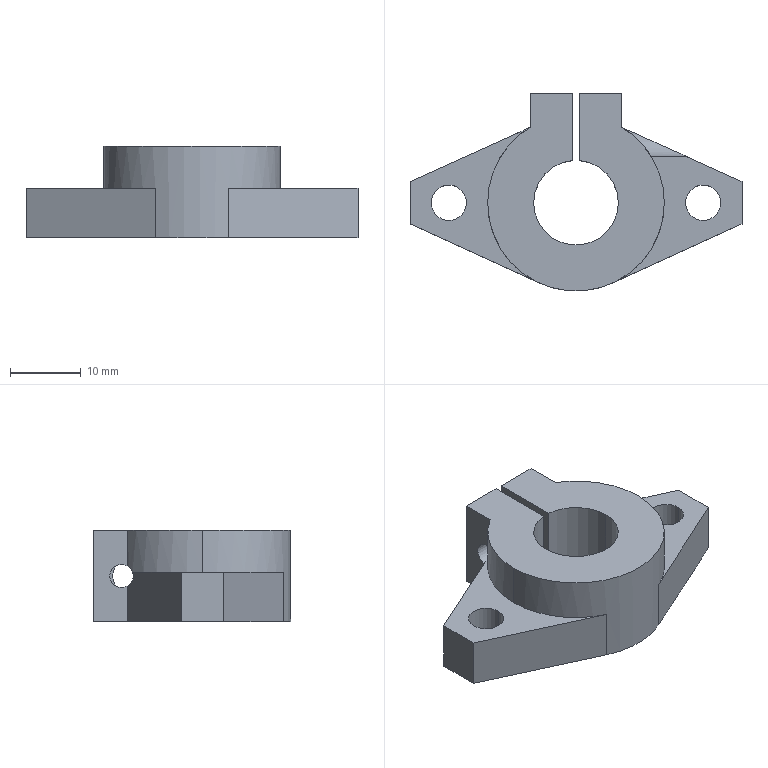Part | SolidWorks | features HoleWzd 2, ICE 2, Extrusion 1 | 1 solid | 33 faces | box 47 x 28 x 13 mm | volume 6727 mm3 | plane 17 | cylinder 16 | commonest cylinder face diameters 5 x4 12 x3 25 x3 3.3 x2 4.5 x2 8 x2
STEP:
#1=CARTESIAN_POINT('',(1.9,10.5,4.));
#2=VERTEX_POINT('',#1);
#3=CARTESIAN_POINT('',(1.9,10.5,-4.));
#4=VERTEX_POINT('',#3);
#5=CARTESIAN_POINT('',(1.9,10.5,0.));
#6=DIRECTION('',(1.,0.,0.));
#7=DIRECTION('',(0.,0.,-1.));
#8=AXIS2_PLACEMENT_3D('',#5,#6,#7);
#9=CIRCLE('',#8,4.);
#10=EDGE_CURVE('',#2,#4,#9,.T.);
#11=ORIENTED_EDGE('',*,*,#10,.F.);
#12=CARTESIAN_POINT('',(6.782,10.5,4.));
#13=VERTEX_POINT('',#12);
#14=CARTESIAN_POINT('',(6.5,10.5,4.));
#15=DIRECTION('',(1.,0.,0.));
#16=VECTOR('',#15,1000.);
#17=LINE('',#14,#16);
#18=EDGE_CURVE('',#2,#13,#17,.T.);
#19=ORIENTED_EDGE('',*,*,#18,.T.);
#20=CARTESIAN_POINT('',(10.658,6.531,0.5));
#21=VERTEX_POINT('',#20);
#22=CARTESIAN_POINT('',(6.782,10.5,4.));
#23=CARTESIAN_POINT('',(7.288,10.174,4.));
#24=CARTESIAN_POINT('',(7.763,9.815,3.961));
#25=CARTESIAN_POINT('',(8.43,9.234,3.8));
#26=CARTESIAN_POINT('',(8.647,9.031,3.727));
#27=CARTESIAN_POINT('',(9.053,8.625,3.54));
#28=CARTESIAN_POINT('',(9.242,8.421,3.426));
#29=CARTESIAN_POINT('',(9.594,8.018,3.146));
#30=CARTESIAN_POINT('',(9.756,7.818,2.979));
#31=CARTESIAN_POINT('',(10.04,7.449,2.601));
#32=CARTESIAN_POINT('',(10.164,7.279,2.388));
#33=CARTESIAN_POINT('',(10.323,7.05,2.028));
#34=CARTESIAN_POINT('',(10.371,6.978,1.902));
#35=CARTESIAN_POINT('',(10.456,6.85,1.642));
#36=CARTESIAN_POINT('',(10.494,6.792,1.508));
#37=CARTESIAN_POINT('',(10.558,6.692,1.233));
#38=CARTESIAN_POINT('',(10.585,6.649,1.091));
#39=CARTESIAN_POINT('',(10.629,6.578,0.7995));
#40=CARTESIAN_POINT('',(10.646,6.55,0.6495));
#41=CARTESIAN_POINT('',(10.658,6.531,0.5));
#42=B_SPLINE_CURVE_WITH_KNOTS('',3,(#22,#23,#24,#25,#26,#27,#28,#29,#30,#31,#32,#33,#34,#35,#36,#37,#38,#39,#40,#41),.UNSPECIFIED.,.F.,.F.,(4,2,2,2,2,2,2,2,2,4),(0.0003296,0.002119,0.003014,0.003908,0.004803,0.005698,0.006145,0.006592,0.00704,0.007487),.UNSPECIFIED.);
#43=EDGE_CURVE('',#13,#21,#42,.T.);
#44=ORIENTED_EDGE('',*,*,#43,.T.);
#45=CARTESIAN_POINT('',(15.68,6.531,0.5));
#46=VERTEX_POINT('',#45);
#47=CARTESIAN_POINT('',(16.5,6.531,0.5));
#48=DIRECTION('',(1.,0.,0.));
#49=VECTOR('',#48,1000.);
#50=LINE('',#47,#49);
#51=EDGE_CURVE('',#21,#46,#50,.T.);
#52=ORIENTED_EDGE('',*,*,#51,.T.);
#53=CARTESIAN_POINT('',(6.892,10.5,-4.));
#54=VERTEX_POINT('',#53);
#55=CARTESIAN_POINT('',(15.68,6.531,0.5));
#56=CARTESIAN_POINT('',(16.395,6.208,-2.063));
#57=CARTESIAN_POINT('',(12.612,7.917,-4.));
#58=CARTESIAN_POINT('',(6.892,10.5,-4.));
#59=(BOUNDED_CURVE()B_SPLINE_CURVE(3,(#55,#56,#57,#58),.UNSPECIFIED.,.F.,.F.)B_SPLINE_CURVE_WITH_KNOTS((4,4),(3.016,4.712),.UNSPECIFIED.)CURVE()GEOMETRIC_REPRESENTATION_ITEM()RATIONAL_B_SPLINE_CURVE((1.,0.7743,0.7743,1.))REPRESENTATION_ITEM(''));
#60=EDGE_CURVE('',#46,#54,#59,.T.);
#61=ORIENTED_EDGE('',*,*,#60,.T.);
#62=CARTESIAN_POINT('',(6.5,10.5,-4.));
#63=DIRECTION('',(1.,0.,0.));
#64=VECTOR('',#63,1000.);
#65=LINE('',#62,#64);
#66=EDGE_CURVE('',#4,#54,#65,.T.);
#67=ORIENTED_EDGE('',*,*,#66,.F.);
#68=EDGE_LOOP('',(#11,#19,#44,#52,#61,#67));
#69=FACE_OUTER_BOUND('',#68,.T.);
#70=CARTESIAN_POINT('',(6.5,10.5,0.));
#71=DIRECTION('',(1.,0.,0.));
#72=DIRECTION('',(0.,0.,-1.));
#73=AXIS2_PLACEMENT_3D('',#70,#71,#72);
#74=CYLINDRICAL_SURFACE('',#73,4.);
#75=ADVANCED_FACE('',(#69),#74,.F.);
#76=CARTESIAN_POINT('',(0.5,10.5,2.25));
#77=VERTEX_POINT('',#76);
#78=CARTESIAN_POINT('',(0.5,10.5,-2.25));
#79=VERTEX_POINT('',#78);
#80=CARTESIAN_POINT('',(0.5,10.5,0.));
#81=DIRECTION('',(1.,0.,0.));
#82=DIRECTION('',(0.,0.,-1.));
#83=AXIS2_PLACEMENT_3D('',#80,#81,#82);
#84=CIRCLE('',#83,2.25);
#85=EDGE_CURVE('',#77,#79,#84,.T.);
#86=ORIENTED_EDGE('',*,*,#85,.F.);
#87=CARTESIAN_POINT('',(1.9,10.5,2.25));
#88=VERTEX_POINT('',#87);
#89=CARTESIAN_POINT('',(6.5,10.5,2.25));
#90=DIRECTION('',(1.,0.,0.));
#91=VECTOR('',#90,1000.);
#92=LINE('',#89,#91);
#93=EDGE_CURVE('',#77,#88,#92,.T.);
#94=ORIENTED_EDGE('',*,*,#93,.T.);
#95=CARTESIAN_POINT('',(1.9,10.5,-2.25));
#96=VERTEX_POINT('',#95);
#97=CARTESIAN_POINT('',(1.9,10.5,0.));
#98=DIRECTION('',(1.,0.,0.));
#99=DIRECTION('',(0.,0.,-1.));
#100=AXIS2_PLACEMENT_3D('',#97,#98,#99);
#101=CIRCLE('',#100,2.25);
#102=EDGE_CURVE('',#88,#96,#101,.T.);
#103=ORIENTED_EDGE('',*,*,#102,.T.);
#104=CARTESIAN_POINT('',(6.5,10.5,-2.25));
#105=DIRECTION('',(1.,0.,0.));
#106=VECTOR('',#105,1000.);
#107=LINE('',#104,#106);
#108=EDGE_CURVE('',#79,#96,#107,.T.);
#109=ORIENTED_EDGE('',*,*,#108,.F.);
#110=EDGE_LOOP('',(#86,#94,#103,#109));
#111=FACE_OUTER_BOUND('',#110,.T.);
#112=CARTESIAN_POINT('',(6.5,10.5,0.));
#113=DIRECTION('',(1.,0.,0.));
#114=DIRECTION('',(0.,0.,-1.));
#115=AXIS2_PLACEMENT_3D('',#112,#113,#114);
#116=CYLINDRICAL_SURFACE('',#115,2.25);
#117=ADVANCED_FACE('',(#111),#116,.F.);
#118=CARTESIAN_POINT('',(-6.5,11.5,1.65));
#119=VERTEX_POINT('',#118);
#120=CARTESIAN_POINT('',(-6.5,10.677,1.43));
#121=VERTEX_POINT('',#120);
#122=CARTESIAN_POINT('',(-6.5,11.5,0.));
#123=DIRECTION('',(1.,0.,0.));
#124=DIRECTION('',(0.,1.,0.));
#125=AXIS2_PLACEMENT_3D('',#122,#123,#124);
#126=CIRCLE('',#125,1.65);
#127=EDGE_CURVE('',#119,#121,#126,.T.);
#128=ORIENTED_EDGE('',*,*,#127,.F.);
#129=CARTESIAN_POINT('',(-0.5,11.5,1.65));
#130=VERTEX_POINT('',#129);
#131=CARTESIAN_POINT('',(-0.5,11.5,1.65));
#132=DIRECTION('',(1.,0.,0.));
#133=VECTOR('',#132,1000.);
#134=LINE('',#131,#133);
#135=EDGE_CURVE('',#119,#130,#134,.T.);
#136=ORIENTED_EDGE('',*,*,#135,.T.);
#137=CARTESIAN_POINT('',(-0.5,11.5,-1.65));
#138=VERTEX_POINT('',#137);
#139=CARTESIAN_POINT('',(-0.5,11.5,0.));
#140=DIRECTION('',(1.,0.,0.));
#141=DIRECTION('',(0.,0.,-1.));
#142=AXIS2_PLACEMENT_3D('',#139,#140,#141);
#143=CIRCLE('',#142,1.65);
#144=EDGE_CURVE('',#130,#138,#143,.T.);
#145=ORIENTED_EDGE('',*,*,#144,.T.);
#146=CARTESIAN_POINT('',(-6.5,11.5,-1.65));
#147=VERTEX_POINT('',#146);
#148=CARTESIAN_POINT('',(-0.5,11.5,-1.65));
#149=DIRECTION('',(1.,0.,0.));
#150=VECTOR('',#149,1000.);
#151=LINE('',#148,#150);
#152=EDGE_CURVE('',#147,#138,#151,.T.);
#153=ORIENTED_EDGE('',*,*,#152,.F.);
#154=CARTESIAN_POINT('',(-6.5,10.677,-1.43));
#155=VERTEX_POINT('',#154);
#156=CARTESIAN_POINT('',(-6.5,11.5,0.));
#157=DIRECTION('',(1.,0.,0.));
#158=DIRECTION('',(0.,1.,0.));
#159=AXIS2_PLACEMENT_3D('',#156,#157,#158);
#160=CIRCLE('',#159,1.65);
#161=EDGE_CURVE('',#155,#147,#160,.T.);
#162=ORIENTED_EDGE('',*,*,#161,.F.);
#163=CARTESIAN_POINT('',(-8.16,9.928,0.5));
#164=VERTEX_POINT('',#163);
#165=CARTESIAN_POINT('',(-6.5,10.677,-1.43));
#166=CARTESIAN_POINT('',(-8.054,9.975,-1.026));
#167=CARTESIAN_POINT('',(-8.703,9.682,-0.2716));
#168=CARTESIAN_POINT('',(-8.16,9.928,0.5));
#169=(BOUNDED_CURVE()B_SPLINE_CURVE(3,(#165,#166,#167,#168),.UNSPECIFIED.,.F.,.F.)B_SPLINE_CURVE_WITH_KNOTS((4,4),(2.093,3.449),.UNSPECIFIED.)CURVE()GEOMETRIC_REPRESENTATION_ITEM()RATIONAL_B_SPLINE_CURVE((1.,0.8524,0.8524,1.))REPRESENTATION_ITEM(''));
#170=EDGE_CURVE('',#155,#164,#169,.T.);
#171=ORIENTED_EDGE('',*,*,#170,.T.);
#172=CARTESIAN_POINT('',(-7.596,9.928,0.5));
#173=VERTEX_POINT('',#172);
#174=CARTESIAN_POINT('',(-0.5,9.928,0.5));
#175=DIRECTION('',(-1.,0.,0.));
#176=VECTOR('',#175,1000.);
#177=LINE('',#174,#176);
#178=EDGE_CURVE('',#173,#164,#177,.T.);
#179=ORIENTED_EDGE('',*,*,#178,.F.);
#180=CARTESIAN_POINT('',(-6.5,10.677,1.43));
#181=CARTESIAN_POINT('',(-6.728,10.538,1.35));
#182=CARTESIAN_POINT('',(-6.941,10.398,1.245));
#183=CARTESIAN_POINT('',(-7.23,10.197,1.018));
#184=CARTESIAN_POINT('',(-7.319,10.134,0.9323));
#185=CARTESIAN_POINT('',(-7.476,10.018,0.7346));
#186=CARTESIAN_POINT('',(-7.544,9.967,0.623));
#187=CARTESIAN_POINT('',(-7.596,9.928,0.5));
#188=B_SPLINE_CURVE_WITH_KNOTS('',3,(#180,#181,#182,#183,#184,#185,#186,#187),.UNSPECIFIED.,.F.,.F.,(4,2,2,4),(0.,0.0008278,0.001242,0.001656),.UNSPECIFIED.);
#189=EDGE_CURVE('',#121,#173,#188,.T.);
#190=ORIENTED_EDGE('',*,*,#189,.F.);
#191=EDGE_LOOP('',(#128,#136,#145,#153,#162,#171,#179,#190));
#192=FACE_OUTER_BOUND('',#191,.T.);
#193=CARTESIAN_POINT('',(-0.5,11.5,0.));
#194=DIRECTION('',(1.,0.,0.));
#195=DIRECTION('',(0.,0.,-1.));
#196=AXIS2_PLACEMENT_3D('',#193,#194,#195);
#197=CYLINDRICAL_SURFACE('',#196,1.65);
#198=ADVANCED_FACE('',(#192),#197,.F.);
#199=CARTESIAN_POINT('',(-15.5,0.,0.5));
#200=VERTEX_POINT('',#199);
#201=CARTESIAN_POINT('',(-20.5,0.,0.5));
#202=VERTEX_POINT('',#201);
#203=CARTESIAN_POINT('',(-18.,0.,0.5));
#204=DIRECTION('',(0.,0.,-1.));
#205=DIRECTION('',(-1.,0.,0.));
#206=AXIS2_PLACEMENT_3D('',#203,#204,#205);
#207=CIRCLE('',#206,2.5);
#208=EDGE_CURVE('',#200,#202,#207,.T.);
#209=ORIENTED_EDGE('',*,*,#208,.F.);
#210=CARTESIAN_POINT('',(-15.5,0.,-6.5));
#211=VERTEX_POINT('',#210);
#212=CARTESIAN_POINT('',(-15.5,0.,0.5));
#213=DIRECTION('',(0.,0.,-1.));
#214=VECTOR('',#213,1000.);
#215=LINE('',#212,#214);
#216=EDGE_CURVE('',#200,#211,#215,.T.);
#217=ORIENTED_EDGE('',*,*,#216,.T.);
#218=CARTESIAN_POINT('',(-20.5,0.,-6.5));
#219=VERTEX_POINT('',#218);
#220=CARTESIAN_POINT('',(-18.,0.,-6.5));
#221=DIRECTION('',(0.,0.,-1.));
#222=DIRECTION('',(-1.,0.,0.));
#223=AXIS2_PLACEMENT_3D('',#220,#221,#222);
#224=CIRCLE('',#223,2.5);
#225=EDGE_CURVE('',#211,#219,#224,.T.);
#226=ORIENTED_EDGE('',*,*,#225,.T.);
#227=CARTESIAN_POINT('',(-20.5,0.,0.5));
#228=DIRECTION('',(0.,0.,-1.));
#229=VECTOR('',#228,1000.);
#230=LINE('',#227,#229);
#231=EDGE_CURVE('',#202,#219,#230,.T.);
#232=ORIENTED_EDGE('',*,*,#231,.F.);
#233=EDGE_LOOP('',(#209,#217,#226,#232));
#234=FACE_OUTER_BOUND('',#233,.T.);
#235=CARTESIAN_POINT('',(-18.,0.,0.5));
#236=DIRECTION('',(0.,0.,-1.));
#237=DIRECTION('',(-1.,0.,0.));
#238=AXIS2_PLACEMENT_3D('',#235,#236,#237);
#239=CYLINDRICAL_SURFACE('',#238,2.5);
#240=ADVANCED_FACE('',(#234),#239,.F.);
#241=CARTESIAN_POINT('',(20.5,0.,0.5));
#242=VERTEX_POINT('',#241);
#243=CARTESIAN_POINT('',(15.5,0.,0.5));
#244=VERTEX_POINT('',#243);
#245=CARTESIAN_POINT('',(18.,0.,0.5));
#246=DIRECTION('',(0.,0.,-1.));
#247=DIRECTION('',(-1.,0.,0.));
#248=AXIS2_PLACEMENT_3D('',#245,#246,#247);
#249=CIRCLE('',#248,2.5);
#250=EDGE_CURVE('',#242,#244,#249,.T.);
#251=ORIENTED_EDGE('',*,*,#250,.F.);
#252=CARTESIAN_POINT('',(20.5,0.,-6.5));
#253=VERTEX_POINT('',#252);
#254=CARTESIAN_POINT('',(20.5,0.,0.5));
#255=DIRECTION('',(0.,0.,-1.));
#256=VECTOR('',#255,1000.);
#257=LINE('',#254,#256);
#258=EDGE_CURVE('',#242,#253,#257,.T.);
#259=ORIENTED_EDGE('',*,*,#258,.T.);
#260=CARTESIAN_POINT('',(15.5,0.,-6.5));
#261=VERTEX_POINT('',#260);
#262=CARTESIAN_POINT('',(18.,0.,-6.5));
#263=DIRECTION('',(0.,0.,-1.));
#264=DIRECTION('',(-1.,0.,0.));
#265=AXIS2_PLACEMENT_3D('',#262,#263,#264);
#266=CIRCLE('',#265,2.5);
#267=EDGE_CURVE('',#253,#261,#266,.T.);
#268=ORIENTED_EDGE('',*,*,#267,.T.);
#269=CARTESIAN_POINT('',(15.5,0.,0.5));
#270=DIRECTION('',(0.,0.,-1.));
#271=VECTOR('',#270,1000.);
#272=LINE('',#269,#271);
#273=EDGE_CURVE('',#244,#261,#272,.T.);
#274=ORIENTED_EDGE('',*,*,#273,.F.);
#275=EDGE_LOOP('',(#251,#259,#268,#274));
#276=FACE_OUTER_BOUND('',#275,.T.);
#277=CARTESIAN_POINT('',(18.,0.,0.5));
#278=DIRECTION('',(0.,0.,-1.));
#279=DIRECTION('',(-1.,0.,0.));
#280=AXIS2_PLACEMENT_3D('',#277,#278,#279);
#281=CYLINDRICAL_SURFACE('',#280,2.5);
#282=ADVANCED_FACE('',(#276),#281,.F.);
#283=CARTESIAN_POINT('',(6.,0.,6.5));
#284=VERTEX_POINT('',#283);
#285=CARTESIAN_POINT('',(-6.,0.,6.5));
#286=VERTEX_POINT('',#285);
#287=CARTESIAN_POINT('',(0.,0.,6.5));
#288=DIRECTION('',(0.,0.,-1.));
#289=DIRECTION('',(1.,0.,0.));
#290=AXIS2_PLACEMENT_3D('',#287,#288,#289);
#291=CIRCLE('',#290,6.);
#292=EDGE_CURVE('',#284,#286,#291,.T.);
#293=ORIENTED_EDGE('',*,*,#292,.F.);
#294=CARTESIAN_POINT('',(6.,0.,-6.5));
#295=VERTEX_POINT('',#294);
#296=CARTESIAN_POINT('',(6.,0.,6.5));
#297=DIRECTION('',(0.,0.,-1.));
#298=VECTOR('',#297,1000.);
#299=LINE('',#296,#298);
#300=EDGE_CURVE('',#284,#295,#299,.T.);
#301=ORIENTED_EDGE('',*,*,#300,.T.);
#302=CARTESIAN_POINT('',(-6.,0.,-6.5));
#303=VERTEX_POINT('',#302);
#304=CARTESIAN_POINT('',(0.,0.,-6.5));
#305=DIRECTION('',(0.,0.,-1.));
#306=DIRECTION('',(1.,0.,0.));
#307=AXIS2_PLACEMENT_3D('',#304,#305,#306);
#308=CIRCLE('',#307,6.);
#309=EDGE_CURVE('',#295,#303,#308,.T.);
#310=ORIENTED_EDGE('',*,*,#309,.T.);
#311=CARTESIAN_POINT('',(-6.,0.,6.5));
#312=DIRECTION('',(0.,0.,-1.));
#313=VECTOR('',#312,1000.);
#314=LINE('',#311,#313);
#315=EDGE_CURVE('',#286,#303,#314,.T.);
#316=ORIENTED_EDGE('',*,*,#315,.F.);
#317=EDGE_LOOP('',(#293,#301,#310,#316));
#318=FACE_OUTER_BOUND('',#317,.T.);
#319=CARTESIAN_POINT('',(0.,0.,6.5));
#320=DIRECTION('',(0.,0.,-1.));
#321=DIRECTION('',(-1.,0.,0.));
#322=AXIS2_PLACEMENT_3D('',#319,#320,#321);
#323=CYLINDRICAL_SURFACE('',#322,6.);
#324=ADVANCED_FACE('',(#318),#323,.F.);
#325=CARTESIAN_POINT('',(-0.5,5.979,6.5));
#326=VERTEX_POINT('',#325);
#327=CARTESIAN_POINT('',(0.,0.,6.5));
#328=DIRECTION('',(0.,0.,-1.));
#329=DIRECTION('',(1.,0.,0.));
#330=AXIS2_PLACEMENT_3D('',#327,#328,#329);
#331=CIRCLE('',#330,6.);
#332=EDGE_CURVE('',#286,#326,#331,.T.);
#333=ORIENTED_EDGE('',*,*,#332,.F.);
#334=ORIENTED_EDGE('',*,*,#315,.T.);
#335=CARTESIAN_POINT('',(-0.5,5.979,-6.5));
#336=VERTEX_POINT('',#335);
#337=CARTESIAN_POINT('',(0.,0.,-6.5));
#338=DIRECTION('',(0.,0.,-1.));
#339=DIRECTION('',(1.,0.,0.));
#340=AXIS2_PLACEMENT_3D('',#337,#338,#339);
#341=CIRCLE('',#340,6.);
#342=EDGE_CURVE('',#303,#336,#341,.T.);
#343=ORIENTED_EDGE('',*,*,#342,.T.);
#344=CARTESIAN_POINT('',(-0.5,5.979,6.5));
#345=DIRECTION('',(0.,0.,-1.));
#346=VECTOR('',#345,1000.);
#347=LINE('',#344,#346);
#348=EDGE_CURVE('',#326,#336,#347,.T.);
#349=ORIENTED_EDGE('',*,*,#348,.F.);
#350=EDGE_LOOP('',(#333,#334,#343,#349));
#351=FACE_OUTER_BOUND('',#350,.T.);
#352=CARTESIAN_POINT('',(0.,0.,6.5));
#353=DIRECTION('',(0.,0.,-1.));
#354=DIRECTION('',(-1.,0.,0.));
#355=AXIS2_PLACEMENT_3D('',#352,#353,#354);
#356=CYLINDRICAL_SURFACE('',#355,6.);
#357=ADVANCED_FACE('',(#351),#356,.F.);
#358=CARTESIAN_POINT('',(12.5,0.,6.5));
#359=VERTEX_POINT('',#358);
#360=CARTESIAN_POINT('',(6.5,10.677,6.5));
#361=VERTEX_POINT('',#360);
#362=CARTESIAN_POINT('',(0.,0.,6.5));
#363=DIRECTION('',(0.,0.,1.));
#364=DIRECTION('',(1.,0.,0.));
#365=AXIS2_PLACEMENT_3D('',#362,#363,#364);
#366=CIRCLE('',#365,12.5);
#367=EDGE_CURVE('',#359,#361,#366,.T.);
#368=ORIENTED_EDGE('',*,*,#367,.F.);
#369=CARTESIAN_POINT('',(12.5,0.,0.5));
#370=VERTEX_POINT('',#369);
#371=CARTESIAN_POINT('',(12.5,0.,6.5));
#372=DIRECTION('',(0.,0.,-1.));
#373=VECTOR('',#372,1000.);
#374=LINE('',#371,#373);
#375=EDGE_CURVE('',#359,#370,#374,.T.);
#376=ORIENTED_EDGE('',*,*,#375,.T.);
#377=CARTESIAN_POINT('',(0.,0.,0.5));
#378=DIRECTION('',(0.,0.,-1.));
#379=DIRECTION('',(-1.,0.,0.));
#380=AXIS2_PLACEMENT_3D('',#377,#378,#379);
#381=CIRCLE('',#380,12.5);
#382=EDGE_CURVE('',#21,#370,#381,.T.);
#383=ORIENTED_EDGE('',*,*,#382,.F.);
#384=ORIENTED_EDGE('',*,*,#43,.F.);
#385=CARTESIAN_POINT('',(6.5,10.677,3.996));
#386=VERTEX_POINT('',#385);
#387=CARTESIAN_POINT('',(6.5,10.677,3.996));
#388=CARTESIAN_POINT('',(6.595,10.619,3.999));
#389=CARTESIAN_POINT('',(6.689,10.56,4.));
#390=CARTESIAN_POINT('',(6.782,10.5,4.));
#391=B_SPLINE_CURVE_WITH_KNOTS('',3,(#387,#388,#389,#390),.UNSPECIFIED.,.F.,.F.,(4,4),(0.,0.0003296),.UNSPECIFIED.);
#392=EDGE_CURVE('',#386,#13,#391,.T.);
#393=ORIENTED_EDGE('',*,*,#392,.F.);
#394=CARTESIAN_POINT('',(6.5,10.677,6.5));
#395=DIRECTION('',(0.,0.,-1.));
#396=VECTOR('',#395,1000.);
#397=LINE('',#394,#396);
#398=EDGE_CURVE('',#361,#386,#397,.T.);
#399=ORIENTED_EDGE('',*,*,#398,.F.);
#400=EDGE_LOOP('',(#368,#376,#383,#384,#393,#399));
#401=FACE_OUTER_BOUND('',#400,.T.);
#402=CARTESIAN_POINT('',(0.,0.,6.5));
#403=DIRECTION('',(0.,0.,-1.));
#404=DIRECTION('',(-1.,0.,0.));
#405=AXIS2_PLACEMENT_3D('',#402,#403,#404);
#406=CYLINDRICAL_SURFACE('',#405,12.5);
#407=ADVANCED_FACE('',(#401),#406,.T.);
#408=ORIENTED_EDGE('',*,*,#375,.F.);
#409=CARTESIAN_POINT('',(-12.5,0.,6.5));
#410=VERTEX_POINT('',#409);
#411=CARTESIAN_POINT('',(0.,0.,6.5));
#412=DIRECTION('',(0.,0.,1.));
#413=DIRECTION('',(1.,0.,0.));
#414=AXIS2_PLACEMENT_3D('',#411,#412,#413);
#415=CIRCLE('',#414,12.5);
#416=EDGE_CURVE('',#410,#359,#415,.T.);
#417=ORIENTED_EDGE('',*,*,#416,.F.);
#418=CARTESIAN_POINT('',(-12.5,0.,0.5));
#419=VERTEX_POINT('',#418);
#420=CARTESIAN_POINT('',(-12.5,0.,6.5));
#421=DIRECTION('',(0.,0.,-1.));
#422=VECTOR('',#421,1000.);
#423=LINE('',#420,#422);
#424=EDGE_CURVE('',#410,#419,#423,.T.);
#425=ORIENTED_EDGE('',*,*,#424,.T.);
#426=CARTESIAN_POINT('',(-5.198,-11.368,0.5));
#427=VERTEX_POINT('',#426);
#428=CARTESIAN_POINT('',(0.,0.,0.5));
#429=DIRECTION('',(0.,0.,-1.));
#430=DIRECTION('',(-1.,0.,0.));
#431=AXIS2_PLACEMENT_3D('',#428,#429,#430);
#432=CIRCLE('',#431,12.5);
#433=EDGE_CURVE('',#427,#419,#432,.T.);
#434=ORIENTED_EDGE('',*,*,#433,.F.);
#435=CARTESIAN_POINT('',(-5.198,-11.368,-6.5));
#436=VERTEX_POINT('',#435);
#437=CARTESIAN_POINT('',(-5.198,-11.368,0.5));
#438=DIRECTION('',(0.,0.,-1.));
#439=VECTOR('',#438,1000.);
#440=LINE('',#437,#439);
#441=EDGE_CURVE('',#427,#436,#440,.T.);
#442=ORIENTED_EDGE('',*,*,#441,.T.);
#443=CARTESIAN_POINT('',(5.198,-11.368,-6.5));
#444=VERTEX_POINT('',#443);
#445=CARTESIAN_POINT('',(0.,0.,-6.5));
#446=DIRECTION('',(0.,0.,1.));
#447=DIRECTION('',(1.,0.,0.));
#448=AXIS2_PLACEMENT_3D('',#445,#446,#447);
#449=CIRCLE('',#448,12.5);
#450=EDGE_CURVE('',#436,#444,#449,.T.);
#451=ORIENTED_EDGE('',*,*,#450,.T.);
#452=CARTESIAN_POINT('',(5.198,-11.368,0.5));
#453=VERTEX_POINT('',#452);
#454=CARTESIAN_POINT('',(5.198,-11.368,0.5));
#455=DIRECTION('',(0.,0.,-1.));
#456=VECTOR('',#455,1000.);
#457=LINE('',#454,#456);
#458=EDGE_CURVE('',#453,#444,#457,.T.);
#459=ORIENTED_EDGE('',*,*,#458,.F.);
#460=CARTESIAN_POINT('',(0.,0.,0.5));
#461=DIRECTION('',(0.,0.,-1.));
#462=DIRECTION('',(-1.,0.,0.));
#463=AXIS2_PLACEMENT_3D('',#460,#461,#462);
#464=CIRCLE('',#463,12.5);
#465=EDGE_CURVE('',#370,#453,#464,.T.);
#466=ORIENTED_EDGE('',*,*,#465,.F.);
#467=EDGE_LOOP('',(#408,#417,#425,#434,#442,#451,#459,#466));
#468=FACE_OUTER_BOUND('',#467,.T.);
#469=CARTESIAN_POINT('',(0.,0.,6.5));
#470=DIRECTION('',(0.,0.,-1.));
#471=DIRECTION('',(-1.,0.,0.));
#472=AXIS2_PLACEMENT_3D('',#469,#470,#471);
#473=CYLINDRICAL_SURFACE('',#472,12.5);
#474=ADVANCED_FACE('',(#468),#473,.T.);
#475=ORIENTED_EDGE('',*,*,#424,.F.);
#476=CARTESIAN_POINT('',(-6.5,10.677,6.5));
#477=VERTEX_POINT('',#476);
#478=CARTESIAN_POINT('',(0.,0.,6.5));
#479=DIRECTION('',(0.,0.,1.));
#480=DIRECTION('',(1.,0.,0.));
#481=AXIS2_PLACEMENT_3D('',#478,#479,#480);
#482=CIRCLE('',#481,12.5);
#483=EDGE_CURVE('',#477,#410,#482,.T.);
#484=ORIENTED_EDGE('',*,*,#483,.F.);
#485=CARTESIAN_POINT('',(-6.5,10.677,6.5));
#486=DIRECTION('',(0.,0.,-1.));
#487=VECTOR('',#486,1000.);
#488=LINE('',#485,#487);
#489=EDGE_CURVE('',#477,#121,#488,.T.);
#490=ORIENTED_EDGE('',*,*,#489,.T.);
#491=ORIENTED_EDGE('',*,*,#189,.T.);
#492=CARTESIAN_POINT('',(0.,0.,0.5));
#493=DIRECTION('',(0.,0.,-1.));
#494=DIRECTION('',(-1.,0.,0.));
#495=AXIS2_PLACEMENT_3D('',#492,#493,#494);
#496=CIRCLE('',#495,12.5);
#497=EDGE_CURVE('',#419,#173,#496,.T.);
#498=ORIENTED_EDGE('',*,*,#497,.F.);
#499=EDGE_LOOP('',(#475,#484,#490,#491,#498));
#500=FACE_OUTER_BOUND('',#499,.T.);
#501=CARTESIAN_POINT('',(0.,0.,6.5));
#502=DIRECTION('',(0.,0.,-1.));
#503=DIRECTION('',(-1.,0.,0.));
#504=AXIS2_PLACEMENT_3D('',#501,#502,#503);
#505=CYLINDRICAL_SURFACE('',#504,12.5);
#506=ADVANCED_FACE('',(#500),#505,.T.);
#507=ORIENTED_EDGE('',*,*,#60,.F.);
#508=CARTESIAN_POINT('',(23.5,3.,0.5));
#509=VERTEX_POINT('',#508);
#510=CARTESIAN_POINT('',(5.106,11.307,0.5));
#511=DIRECTION('',(-0.9114,0.4116,0.));
#512=VECTOR('',#511,1000.);
#513=LINE('',#510,#512);
#514=EDGE_CURVE('',#509,#46,#513,.T.);
#515=ORIENTED_EDGE('',*,*,#514,.F.);
#516=CARTESIAN_POINT('',(23.5,3.,-6.5));
#517=VERTEX_POINT('',#516);
#518=CARTESIAN_POINT('',(23.5,3.,0.5));
#519=DIRECTION('',(0.,0.,-1.));
#520=VECTOR('',#519,1000.);
#521=LINE('',#518,#520);
#522=EDGE_CURVE('',#509,#517,#521,.T.);
#523=ORIENTED_EDGE('',*,*,#522,.T.);
#524=CARTESIAN_POINT('',(6.5,10.677,-6.5));
#525=VERTEX_POINT('',#524);
#526=CARTESIAN_POINT('',(5.106,11.307,-6.5));
#527=DIRECTION('',(-0.9114,0.4116,0.));
#528=VECTOR('',#527,1000.);
#529=LINE('',#526,#528);
#530=EDGE_CURVE('',#517,#525,#529,.T.);
#531=ORIENTED_EDGE('',*,*,#530,.T.);
#532=CARTESIAN_POINT('',(6.5,10.677,-3.996));
#533=VERTEX_POINT('',#532);
#534=CARTESIAN_POINT('',(6.5,10.677,0.5));
#535=DIRECTION('',(0.,0.,-1.));
#536=VECTOR('',#535,1000.);
#537=LINE('',#534,#536);
#538=EDGE_CURVE('',#533,#525,#537,.T.);
#539=ORIENTED_EDGE('',*,*,#538,.F.);
#540=CARTESIAN_POINT('',(6.892,10.5,-4.));
#541=CARTESIAN_POINT('',(6.761,10.559,-4.));
#542=CARTESIAN_POINT('',(6.631,10.618,-3.999));
#543=CARTESIAN_POINT('',(6.5,10.677,-3.996));
#544=(BOUNDED_CURVE()B_SPLINE_CURVE(3,(#540,#541,#542,#543),.UNSPECIFIED.,.F.,.F.)B_SPLINE_CURVE_WITH_KNOTS((4,4),(4.712,4.757),.UNSPECIFIED.)CURVE()GEOMETRIC_REPRESENTATION_ITEM()RATIONAL_B_SPLINE_CURVE((1.,0.9998,0.9998,1.))REPRESENTATION_ITEM(''));
#545=EDGE_CURVE('',#54,#533,#544,.T.);
#546=ORIENTED_EDGE('',*,*,#545,.F.);
#547=EDGE_LOOP('',(#507,#515,#523,#531,#539,#546));
#548=FACE_OUTER_BOUND('',#547,.T.);
#549=CARTESIAN_POINT('',(5.106,11.307,0.5));
#550=DIRECTION('',(-0.4116,-0.9114,0.));
#551=DIRECTION('',(0.9114,-0.4116,0.));
#552=AXIS2_PLACEMENT_3D('',#549,#550,#551);
#553=PLANE('',#552);
#554=ADVANCED_FACE('',(#548),#553,.F.);
#555=CARTESIAN_POINT('',(18.,0.,0.5));
#556=DIRECTION('',(0.,0.,-1.));
#557=DIRECTION('',(-1.,0.,0.));
#558=AXIS2_PLACEMENT_3D('',#555,#556,#557);
#559=CIRCLE('',#558,2.5);
#560=EDGE_CURVE('',#244,#242,#559,.T.);
#561=ORIENTED_EDGE('',*,*,#560,.T.);
#562=ORIENTED_EDGE('',*,*,#250,.T.);
#563=EDGE_LOOP('',(#561,#562));
#564=FACE_BOUND('',#563,.T.);
#565=ORIENTED_EDGE('',*,*,#51,.F.);
#566=ORIENTED_EDGE('',*,*,#382,.T.);
#567=ORIENTED_EDGE('',*,*,#465,.T.);
#568=CARTESIAN_POINT('',(23.5,-3.,0.5));
#569=VERTEX_POINT('',#568);
#570=CARTESIAN_POINT('',(5.198,-11.368,0.5));
#571=DIRECTION('',(0.9094,0.4158,0.));
#572=VECTOR('',#571,1000.);
#573=LINE('',#570,#572);
#574=EDGE_CURVE('',#453,#569,#573,.T.);
#575=ORIENTED_EDGE('',*,*,#574,.T.);
#576=CARTESIAN_POINT('',(23.5,0.,0.5));
#577=DIRECTION('',(0.,1.,0.));
#578=VECTOR('',#577,1000.);
#579=LINE('',#576,#578);
#580=EDGE_CURVE('',#569,#509,#579,.T.);
#581=ORIENTED_EDGE('',*,*,#580,.T.);
#582=ORIENTED_EDGE('',*,*,#514,.T.);
#583=EDGE_LOOP('',(#565,#566,#567,#575,#581,#582));
#584=FACE_OUTER_BOUND('',#583,.T.);
#585=CARTESIAN_POINT('',(0.,0.,0.5));
#586=DIRECTION('',(0.,0.,-1.));
#587=DIRECTION('',(-1.,0.,0.));
#588=AXIS2_PLACEMENT_3D('',#585,#586,#587);
#589=PLANE('',#588);
#590=ADVANCED_FACE('',(#564,#584),#589,.F.);
#591=ORIENTED_EDGE('',*,*,#300,.F.);
#592=CARTESIAN_POINT('',(0.5,5.979,6.5));
#593=VERTEX_POINT('',#592);
#594=CARTESIAN_POINT('',(0.,0.,6.5));
#595=DIRECTION('',(0.,0.,-1.));
#596=DIRECTION('',(1.,0.,0.));
#597=AXIS2_PLACEMENT_3D('',#594,#595,#596);
#598=CIRCLE('',#597,6.);
#599=EDGE_CURVE('',#593,#284,#598,.T.);
#600=ORIENTED_EDGE('',*,*,#599,.F.);
#601=CARTESIAN_POINT('',(0.5,5.979,-6.5));
#602=VERTEX_POINT('',#601);
#603=CARTESIAN_POINT('',(0.5,5.979,6.5));
#604=DIRECTION('',(0.,0.,-1.));
#605=VECTOR('',#604,1000.);
#606=LINE('',#603,#605);
#607=EDGE_CURVE('',#593,#602,#606,.T.);
#608=ORIENTED_EDGE('',*,*,#607,.T.);
#609=CARTESIAN_POINT('',(0.,0.,-6.5));
#610=DIRECTION('',(0.,0.,-1.));
#611=DIRECTION('',(1.,0.,0.));
#612=AXIS2_PLACEMENT_3D('',#609,#610,#611);
#613=CIRCLE('',#612,6.);
#614=EDGE_CURVE('',#602,#295,#613,.T.);
#615=ORIENTED_EDGE('',*,*,#614,.T.);
#616=EDGE_LOOP('',(#591,#600,#608,#615));
#617=FACE_OUTER_BOUND('',#616,.T.);
#618=CARTESIAN_POINT('',(0.,0.,6.5));
#619=DIRECTION('',(0.,0.,-1.));
#620=DIRECTION('',(-1.,0.,0.));
#621=AXIS2_PLACEMENT_3D('',#618,#619,#620);
#622=CYLINDRICAL_SURFACE('',#621,6.);
#623=ADVANCED_FACE('',(#617),#622,.F.);
#624=CARTESIAN_POINT('',(-0.5,11.5,0.));
#625=DIRECTION('',(1.,0.,0.));
#626=DIRECTION('',(0.,0.,-1.));
#627=AXIS2_PLACEMENT_3D('',#624,#625,#626);
#628=CIRCLE('',#627,1.65);
#629=EDGE_CURVE('',#138,#130,#628,.T.);
#630=ORIENTED_EDGE('',*,*,#629,.F.);
#631=ORIENTED_EDGE('',*,*,#144,.F.);
#632=EDGE_LOOP('',(#630,#631));
#633=FACE_BOUND('',#632,.T.);
#634=CARTESIAN_POINT('',(-0.5,15.5,-6.5));
#635=VERTEX_POINT('',#634);
#636=CARTESIAN_POINT('',(-0.5,5.979,-6.5));
#637=DIRECTION('',(0.,1.,0.));
#638=VECTOR('',#637,1000.);
#639=LINE('',#636,#638);
#640=EDGE_CURVE('',#336,#635,#639,.T.);
#641=ORIENTED_EDGE('',*,*,#640,.T.);
#642=CARTESIAN_POINT('',(-0.5,15.5,6.5));
#643=VERTEX_POINT('',#642);
#644=CARTESIAN_POINT('',(-0.5,15.5,6.5));
#645=DIRECTION('',(0.,0.,-1.));
#646=VECTOR('',#645,1000.);
#647=LINE('',#644,#646);
#648=EDGE_CURVE('',#643,#635,#647,.T.);
#649=ORIENTED_EDGE('',*,*,#648,.F.);
#650=CARTESIAN_POINT('',(-0.5,5.979,6.5));
#651=DIRECTION('',(0.,1.,0.));
#652=VECTOR('',#651,1000.);
#653=LINE('',#650,#652);
#654=EDGE_CURVE('',#326,#643,#653,.T.);
#655=ORIENTED_EDGE('',*,*,#654,.F.);
#656=ORIENTED_EDGE('',*,*,#348,.T.);
#657=EDGE_LOOP('',(#641,#649,#655,#656));
#658=FACE_OUTER_BOUND('',#657,.T.);
#659=CARTESIAN_POINT('',(-0.5,5.979,6.5));
#660=DIRECTION('',(-1.,0.,0.));
#661=DIRECTION('',(0.,-1.,0.));
#662=AXIS2_PLACEMENT_3D('',#659,#660,#661);
#663=PLANE('',#662);
#664=ADVANCED_FACE('',(#633,#658),#663,.F.);
#665=CARTESIAN_POINT('',(-6.5,15.5,-6.5));
#666=VERTEX_POINT('',#665);
#667=CARTESIAN_POINT('',(-6.5,15.5,-6.5));
#668=DIRECTION('',(-1.,0.,0.));
#669=VECTOR('',#668,1000.);
#670=LINE('',#667,#669);
#671=EDGE_CURVE('',#635,#666,#670,.T.);
#672=ORIENTED_EDGE('',*,*,#671,.T.);
#673=CARTESIAN_POINT('',(-6.5,15.5,6.5));
#674=VERTEX_POINT('',#673);
#675=CARTESIAN_POINT('',(-6.5,15.5,6.5));
#676=DIRECTION('',(0.,0.,-1.));
#677=VECTOR('',#676,1000.);
#678=LINE('',#675,#677);
#679=EDGE_CURVE('',#674,#666,#678,.T.);
#680=ORIENTED_EDGE('',*,*,#679,.F.);
#681=CARTESIAN_POINT('',(-6.5,15.5,6.5));
#682=DIRECTION('',(-1.,0.,0.));
#683=VECTOR('',#682,1000.);
#684=LINE('',#681,#683);
#685=EDGE_CURVE('',#643,#674,#684,.T.);
#686=ORIENTED_EDGE('',*,*,#685,.F.);
#687=ORIENTED_EDGE('',*,*,#648,.T.);
#688=EDGE_LOOP('',(#672,#680,#686,#687));
#689=FACE_OUTER_BOUND('',#688,.T.);
#690=CARTESIAN_POINT('',(-6.5,15.5,6.5));
#691=DIRECTION('',(0.,-1.,0.));
#692=DIRECTION('',(0.,0.,-1.));
#693=AXIS2_PLACEMENT_3D('',#690,#691,#692);
#694=PLANE('',#693);
#695=ADVANCED_FACE('',(#689),#694,.F.);
#696=CARTESIAN_POINT('',(-6.5,10.677,-6.5));
#697=VERTEX_POINT('',#696);
#698=CARTESIAN_POINT('',(-6.5,10.677,0.5));
#699=DIRECTION('',(0.,0.,-1.));
#700=VECTOR('',#699,1000.);
#701=LINE('',#698,#700);
#702=EDGE_CURVE('',#155,#697,#701,.T.);
#703=ORIENTED_EDGE('',*,*,#702,.F.);
#704=ORIENTED_EDGE('',*,*,#161,.T.);
#705=CARTESIAN_POINT('',(-6.5,11.5,0.));
#706=DIRECTION('',(1.,0.,0.));
#707=DIRECTION('',(0.,1.,0.));
#708=AXIS2_PLACEMENT_3D('',#705,#706,#707);
#709=CIRCLE('',#708,1.65);
#710=EDGE_CURVE('',#147,#119,#709,.T.);
#711=ORIENTED_EDGE('',*,*,#710,.T.);
#712=ORIENTED_EDGE('',*,*,#127,.T.);
#713=ORIENTED_EDGE('',*,*,#489,.F.);
#714=CARTESIAN_POINT('',(-6.5,15.5,6.5));
#715=DIRECTION('',(0.,-1.,0.));
#716=VECTOR('',#715,1000.);
#717=LINE('',#714,#716);
#718=EDGE_CURVE('',#674,#477,#717,.T.);
#719=ORIENTED_EDGE('',*,*,#718,.F.);
#720=ORIENTED_EDGE('',*,*,#679,.T.);
#721=CARTESIAN_POINT('',(-6.5,15.5,-6.5));
#722=DIRECTION('',(0.,-1.,0.));
#723=VECTOR('',#722,1000.);
#724=LINE('',#721,#723);
#725=EDGE_CURVE('',#666,#697,#724,.T.);
#726=ORIENTED_EDGE('',*,*,#725,.T.);
#727=EDGE_LOOP('',(#703,#704,#711,#712,#713,#719,#720,#726));
#728=FACE_OUTER_BOUND('',#727,.T.);
#729=CARTESIAN_POINT('',(-6.5,15.5,6.5));
#730=DIRECTION('',(1.,0.,0.));
#731=DIRECTION('',(0.,1.,0.));
#732=AXIS2_PLACEMENT_3D('',#729,#730,#731);
#733=PLANE('',#732);
#734=ADVANCED_FACE('',(#728),#733,.F.);
#735=ORIENTED_EDGE('',*,*,#398,.T.);
#736=CARTESIAN_POINT('',(6.5,10.5,0.));
#737=DIRECTION('',(1.,0.,0.));
#738=DIRECTION('',(0.,0.,-1.));
#739=AXIS2_PLACEMENT_3D('',#736,#737,#738);
#740=CIRCLE('',#739,4.);
#741=EDGE_CURVE('',#533,#386,#740,.T.);
#742=ORIENTED_EDGE('',*,*,#741,.F.);
#743=ORIENTED_EDGE('',*,*,#538,.T.);
#744=CARTESIAN_POINT('',(6.5,15.5,-6.5));
#745=VERTEX_POINT('',#744);
#746=CARTESIAN_POINT('',(6.5,15.5,-6.5));
#747=DIRECTION('',(0.,1.,0.));
#748=VECTOR('',#747,1000.);
#749=LINE('',#746,#748);
#750=EDGE_CURVE('',#525,#745,#749,.T.);
#751=ORIENTED_EDGE('',*,*,#750,.T.);
#752=CARTESIAN_POINT('',(6.5,15.5,6.5));
#753=VERTEX_POINT('',#752);
#754=CARTESIAN_POINT('',(6.5,15.5,6.5));
#755=DIRECTION('',(0.,0.,-1.));
#756=VECTOR('',#755,1000.);
#757=LINE('',#754,#756);
#758=EDGE_CURVE('',#753,#745,#757,.T.);
#759=ORIENTED_EDGE('',*,*,#758,.F.);
#760=CARTESIAN_POINT('',(6.5,15.5,6.5));
#761=DIRECTION('',(0.,1.,0.));
#762=VECTOR('',#761,1000.);
#763=LINE('',#760,#762);
#764=EDGE_CURVE('',#361,#753,#763,.T.);
#765=ORIENTED_EDGE('',*,*,#764,.F.);
#766=EDGE_LOOP('',(#735,#742,#743,#751,#759,#765));
#767=FACE_OUTER_BOUND('',#766,.T.);
#768=CARTESIAN_POINT('',(6.5,15.5,6.5));
#769=DIRECTION('',(-1.,0.,0.));
#770=DIRECTION('',(0.,0.,1.));
#771=AXIS2_PLACEMENT_3D('',#768,#769,#770);
#772=PLANE('',#771);
#773=ADVANCED_FACE('',(#767),#772,.F.);
#774=CARTESIAN_POINT('',(0.5,15.5,-6.5));
#775=VERTEX_POINT('',#774);
#776=CARTESIAN_POINT('',(0.5,15.5,-6.5));
#777=DIRECTION('',(-1.,0.,0.));
#778=VECTOR('',#777,1000.);
#779=LINE('',#776,#778);
#780=EDGE_CURVE('',#745,#775,#779,.T.);
#781=ORIENTED_EDGE('',*,*,#780,.T.);
#782=CARTESIAN_POINT('',(0.5,15.5,6.5));
#783=VERTEX_POINT('',#782);
#784=CARTESIAN_POINT('',(0.5,15.5,6.5));
#785=DIRECTION('',(0.,0.,-1.));
#786=VECTOR('',#785,1000.);
#787=LINE('',#784,#786);
#788=EDGE_CURVE('',#783,#775,#787,.T.);
#789=ORIENTED_EDGE('',*,*,#788,.F.);
#790=CARTESIAN_POINT('',(0.5,15.5,6.5));
#791=DIRECTION('',(-1.,0.,0.));
#792=VECTOR('',#791,1000.);
#793=LINE('',#790,#792);
#794=EDGE_CURVE('',#753,#783,#793,.T.);
#795=ORIENTED_EDGE('',*,*,#794,.F.);
#796=ORIENTED_EDGE('',*,*,#758,.T.);
#797=EDGE_LOOP('',(#781,#789,#795,#796));
#798=FACE_OUTER_BOUND('',#797,.T.);
#799=CARTESIAN_POINT('',(0.5,15.5,6.5));
#800=DIRECTION('',(0.,-1.,0.));
#801=DIRECTION('',(0.,0.,-1.));
#802=AXIS2_PLACEMENT_3D('',#799,#800,#801);
#803=PLANE('',#802);
#804=ADVANCED_FACE('',(#798),#803,.F.);
#805=CARTESIAN_POINT('',(0.5,10.5,0.));
#806=DIRECTION('',(1.,0.,0.));
#807=DIRECTION('',(0.,0.,-1.));
#808=AXIS2_PLACEMENT_3D('',#805,#806,#807);
#809=CIRCLE('',#808,2.25);
#810=EDGE_CURVE('',#79,#77,#809,.T.);
#811=ORIENTED_EDGE('',*,*,#810,.T.);
#812=ORIENTED_EDGE('',*,*,#85,.T.);
#813=EDGE_LOOP('',(#811,#812));
#814=FACE_BOUND('',#813,.T.);
#815=CARTESIAN_POINT('',(0.5,5.979,-6.5));
#816=DIRECTION('',(0.,-1.,0.));
#817=VECTOR('',#816,1000.);
#818=LINE('',#815,#817);
#819=EDGE_CURVE('',#775,#602,#818,.T.);
#820=ORIENTED_EDGE('',*,*,#819,.T.);
#821=ORIENTED_EDGE('',*,*,#607,.F.);
#822=CARTESIAN_POINT('',(0.5,5.979,6.5));
#823=DIRECTION('',(0.,-1.,0.));
#824=VECTOR('',#823,1000.);
#825=LINE('',#822,#824);
#826=EDGE_CURVE('',#783,#593,#825,.T.);
#827=ORIENTED_EDGE('',*,*,#826,.F.);
#828=ORIENTED_EDGE('',*,*,#788,.T.);
#829=EDGE_LOOP('',(#820,#821,#827,#828));
#830=FACE_OUTER_BOUND('',#829,.T.);
#831=CARTESIAN_POINT('',(0.5,5.979,6.5));
#832=DIRECTION('',(1.,0.,0.));
#833=DIRECTION('',(0.,0.,-1.));
#834=AXIS2_PLACEMENT_3D('',#831,#832,#833);
#835=PLANE('',#834);
#836=ADVANCED_FACE('',(#814,#830),#835,.F.);
#837=ORIENTED_EDGE('',*,*,#599,.T.);
#838=ORIENTED_EDGE('',*,*,#292,.T.);
#839=ORIENTED_EDGE('',*,*,#332,.T.);
#840=ORIENTED_EDGE('',*,*,#654,.T.);
#841=ORIENTED_EDGE('',*,*,#685,.T.);
#842=ORIENTED_EDGE('',*,*,#718,.T.);
#843=ORIENTED_EDGE('',*,*,#483,.T.);
#844=ORIENTED_EDGE('',*,*,#416,.T.);
#845=ORIENTED_EDGE('',*,*,#367,.T.);
#846=ORIENTED_EDGE('',*,*,#764,.T.);
#847=ORIENTED_EDGE('',*,*,#794,.T.);
#848=ORIENTED_EDGE('',*,*,#826,.T.);
#849=EDGE_LOOP('',(#837,#838,#839,#840,#841,#842,#843,#844,#845,#846,#847,#848));
#850=FACE_OUTER_BOUND('',#849,.T.);
#851=CARTESIAN_POINT('',(0.,0.,6.5));
#852=DIRECTION('',(0.,0.,1.));
#853=DIRECTION('',(1.,0.,0.));
#854=AXIS2_PLACEMENT_3D('',#851,#852,#853);
#855=PLANE('',#854);
#856=ADVANCED_FACE('',(#850),#855,.T.);
#857=ORIENTED_EDGE('',*,*,#614,.F.);
#858=ORIENTED_EDGE('',*,*,#819,.F.);
#859=ORIENTED_EDGE('',*,*,#780,.F.);
#860=ORIENTED_EDGE('',*,*,#750,.F.);
#861=ORIENTED_EDGE('',*,*,#530,.F.);
#862=CARTESIAN_POINT('',(23.5,-3.,-6.5));
#863=VERTEX_POINT('',#862);
#864=CARTESIAN_POINT('',(23.5,0.,-6.5));
#865=DIRECTION('',(0.,1.,0.));
#866=VECTOR('',#865,1000.);
#867=LINE('',#864,#866);
#868=EDGE_CURVE('',#863,#517,#867,.T.);
#869=ORIENTED_EDGE('',*,*,#868,.F.);
#870=CARTESIAN_POINT('',(5.198,-11.368,-6.5));
#871=DIRECTION('',(0.9094,0.4158,0.));
#872=VECTOR('',#871,1000.);
#873=LINE('',#870,#872);
#874=EDGE_CURVE('',#444,#863,#873,.T.);
#875=ORIENTED_EDGE('',*,*,#874,.F.);
#876=ORIENTED_EDGE('',*,*,#450,.F.);
#877=CARTESIAN_POINT('',(-23.5,-3.,-6.5));
#878=VERTEX_POINT('',#877);
#879=CARTESIAN_POINT('',(-5.198,-11.368,-6.5));
#880=DIRECTION('',(-0.9094,0.4158,0.));
#881=VECTOR('',#880,1000.);
#882=LINE('',#879,#881);
#883=EDGE_CURVE('',#436,#878,#882,.T.);
#884=ORIENTED_EDGE('',*,*,#883,.T.);
#885=CARTESIAN_POINT('',(-23.5,3.,-6.5));
#886=VERTEX_POINT('',#885);
#887=CARTESIAN_POINT('',(-23.5,0.,-6.5));
#888=DIRECTION('',(0.,1.,0.));
#889=VECTOR('',#888,1000.);
#890=LINE('',#887,#889);
#891=EDGE_CURVE('',#878,#886,#890,.T.);
#892=ORIENTED_EDGE('',*,*,#891,.T.);
#893=CARTESIAN_POINT('',(-5.106,11.307,-6.5));
#894=DIRECTION('',(0.9114,0.4116,0.));
#895=VECTOR('',#894,1000.);
#896=LINE('',#893,#895);
#897=EDGE_CURVE('',#886,#697,#896,.T.);
#898=ORIENTED_EDGE('',*,*,#897,.T.);
#899=ORIENTED_EDGE('',*,*,#725,.F.);
#900=ORIENTED_EDGE('',*,*,#671,.F.);
#901=ORIENTED_EDGE('',*,*,#640,.F.);
#902=ORIENTED_EDGE('',*,*,#342,.F.);
#903=ORIENTED_EDGE('',*,*,#309,.F.);
#904=EDGE_LOOP('',(#857,#858,#859,#860,#861,#869,#875,#876,#884,#892,#898,#899,#900,#901,#902,#903));
#905=FACE_OUTER_BOUND('',#904,.T.);
#906=CARTESIAN_POINT('',(18.,0.,-6.5));
#907=DIRECTION('',(0.,0.,-1.));
#908=DIRECTION('',(-1.,0.,0.));
#909=AXIS2_PLACEMENT_3D('',#906,#907,#908);
#910=CIRCLE('',#909,2.5);
#911=EDGE_CURVE('',#261,#253,#910,.T.);
#912=ORIENTED_EDGE('',*,*,#911,.F.);
#913=ORIENTED_EDGE('',*,*,#267,.F.);
#914=EDGE_LOOP('',(#912,#913));
#915=FACE_BOUND('',#914,.T.);
#916=CARTESIAN_POINT('',(-18.,0.,-6.5));
#917=DIRECTION('',(0.,0.,-1.));
#918=DIRECTION('',(-1.,0.,0.));
#919=AXIS2_PLACEMENT_3D('',#916,#917,#918);
#920=CIRCLE('',#919,2.5);
#921=EDGE_CURVE('',#219,#211,#920,.T.);
#922=ORIENTED_EDGE('',*,*,#921,.F.);
#923=ORIENTED_EDGE('',*,*,#225,.F.);
#924=EDGE_LOOP('',(#922,#923));
#925=FACE_BOUND('',#924,.T.);
#926=CARTESIAN_POINT('',(0.,0.,-6.5));
#927=DIRECTION('',(0.,0.,1.));
#928=DIRECTION('',(1.,0.,0.));
#929=AXIS2_PLACEMENT_3D('',#926,#927,#928);
#930=PLANE('',#929);
#931=ADVANCED_FACE('',(#905,#915,#925),#930,.F.);
#932=ORIENTED_EDGE('',*,*,#874,.T.);
#933=CARTESIAN_POINT('',(23.5,-3.,0.5));
#934=DIRECTION('',(0.,0.,-1.));
#935=VECTOR('',#934,1000.);
#936=LINE('',#933,#935);
#937=EDGE_CURVE('',#569,#863,#936,.T.);
#938=ORIENTED_EDGE('',*,*,#937,.F.);
#939=ORIENTED_EDGE('',*,*,#574,.F.);
#940=ORIENTED_EDGE('',*,*,#458,.T.);
#941=EDGE_LOOP('',(#932,#938,#939,#940));
#942=FACE_OUTER_BOUND('',#941,.T.);
#943=CARTESIAN_POINT('',(5.198,-11.368,0.5));
#944=DIRECTION('',(-0.4158,0.9094,0.));
#945=DIRECTION('',(-0.9094,-0.4158,0.));
#946=AXIS2_PLACEMENT_3D('',#943,#944,#945);
#947=PLANE('',#946);
#948=ADVANCED_FACE('',(#942),#947,.F.);
#949=ORIENTED_EDGE('',*,*,#258,.F.);
#950=ORIENTED_EDGE('',*,*,#560,.F.);
#951=ORIENTED_EDGE('',*,*,#273,.T.);
#952=ORIENTED_EDGE('',*,*,#911,.T.);
#953=EDGE_LOOP('',(#949,#950,#951,#952));
#954=FACE_OUTER_BOUND('',#953,.T.);
#955=CARTESIAN_POINT('',(18.,0.,0.5));
#956=DIRECTION('',(0.,0.,-1.));
#957=DIRECTION('',(-1.,0.,0.));
#958=AXIS2_PLACEMENT_3D('',#955,#956,#957);
#959=CYLINDRICAL_SURFACE('',#958,2.5);
#960=ADVANCED_FACE('',(#954),#959,.F.);
#961=ORIENTED_EDGE('',*,*,#868,.T.);
#962=ORIENTED_EDGE('',*,*,#522,.F.);
#963=ORIENTED_EDGE('',*,*,#580,.F.);
#964=ORIENTED_EDGE('',*,*,#937,.T.);
#965=EDGE_LOOP('',(#961,#962,#963,#964));
#966=FACE_OUTER_BOUND('',#965,.T.);
#967=CARTESIAN_POINT('',(23.5,0.,0.5));
#968=DIRECTION('',(-1.,0.,0.));
#969=DIRECTION('',(0.,0.,1.));
#970=AXIS2_PLACEMENT_3D('',#967,#968,#969);
#971=PLANE('',#970);
#972=ADVANCED_FACE('',(#966),#971,.F.);
#973=ORIENTED_EDGE('',*,*,#891,.F.);
#974=CARTESIAN_POINT('',(-23.5,-3.,0.5));
#975=VERTEX_POINT('',#974);
#976=CARTESIAN_POINT('',(-23.5,-3.,0.5));
#977=DIRECTION('',(0.,0.,-1.));
#978=VECTOR('',#977,1000.);
#979=LINE('',#976,#978);
#980=EDGE_CURVE('',#975,#878,#979,.T.);
#981=ORIENTED_EDGE('',*,*,#980,.F.);
#982=CARTESIAN_POINT('',(-23.5,3.,0.5));
#983=VERTEX_POINT('',#982);
#984=CARTESIAN_POINT('',(-23.5,0.,0.5));
#985=DIRECTION('',(0.,1.,0.));
#986=VECTOR('',#985,1000.);
#987=LINE('',#984,#986);
#988=EDGE_CURVE('',#975,#983,#987,.T.);
#989=ORIENTED_EDGE('',*,*,#988,.T.);
#990=CARTESIAN_POINT('',(-23.5,3.,0.5));
#991=DIRECTION('',(0.,0.,-1.));
#992=VECTOR('',#991,1000.);
#993=LINE('',#990,#992);
#994=EDGE_CURVE('',#983,#886,#993,.T.);
#995=ORIENTED_EDGE('',*,*,#994,.T.);
#996=EDGE_LOOP('',(#973,#981,#989,#995));
#997=FACE_OUTER_BOUND('',#996,.T.);
#998=CARTESIAN_POINT('',(-23.5,0.,0.5));
#999=DIRECTION('',(-1.,0.,0.));
#1000=DIRECTION('',(0.,0.,1.));
#1001=AXIS2_PLACEMENT_3D('',#998,#999,#1000);
#1002=PLANE('',#1001);
#1003=ADVANCED_FACE('',(#997),#1002,.T.);
#1004=ORIENTED_EDGE('',*,*,#883,.F.);
#1005=ORIENTED_EDGE('',*,*,#441,.F.);
#1006=CARTESIAN_POINT('',(-5.198,-11.368,0.5));
#1007=DIRECTION('',(-0.9094,0.4158,0.));
#1008=VECTOR('',#1007,1000.);
#1009=LINE('',#1006,#1008);
#1010=EDGE_CURVE('',#427,#975,#1009,.T.);
#1011=ORIENTED_EDGE('',*,*,#1010,.T.);
#1012=ORIENTED_EDGE('',*,*,#980,.T.);
#1013=EDGE_LOOP('',(#1004,#1005,#1011,#1012));
#1014=FACE_OUTER_BOUND('',#1013,.T.);
#1015=CARTESIAN_POINT('',(-5.198,-11.368,0.5));
#1016=DIRECTION('',(-0.4158,-0.9094,0.));
#1017=DIRECTION('',(0.9094,-0.4158,0.));
#1018=AXIS2_PLACEMENT_3D('',#1015,#1016,#1017);
#1019=PLANE('',#1018);
#1020=ADVANCED_FACE('',(#1014),#1019,.T.);
#1021=ORIENTED_EDGE('',*,*,#216,.F.);
#1022=CARTESIAN_POINT('',(-18.,0.,0.5));
#1023=DIRECTION('',(0.,0.,-1.));
#1024=DIRECTION('',(-1.,0.,0.));
#1025=AXIS2_PLACEMENT_3D('',#1022,#1023,#1024);
#1026=CIRCLE('',#1025,2.5);
#1027=EDGE_CURVE('',#202,#200,#1026,.T.);
#1028=ORIENTED_EDGE('',*,*,#1027,.F.);
#1029=ORIENTED_EDGE('',*,*,#231,.T.);
#1030=ORIENTED_EDGE('',*,*,#921,.T.);
#1031=EDGE_LOOP('',(#1021,#1028,#1029,#1030));
#1032=FACE_OUTER_BOUND('',#1031,.T.);
#1033=CARTESIAN_POINT('',(-18.,0.,0.5));
#1034=DIRECTION('',(0.,0.,-1.));
#1035=DIRECTION('',(-1.,0.,0.));
#1036=AXIS2_PLACEMENT_3D('',#1033,#1034,#1035);
#1037=CYLINDRICAL_SURFACE('',#1036,2.5);
#1038=ADVANCED_FACE('',(#1032),#1037,.F.);
#1039=ORIENTED_EDGE('',*,*,#170,.F.);
#1040=ORIENTED_EDGE('',*,*,#702,.T.);
#1041=ORIENTED_EDGE('',*,*,#897,.F.);
#1042=ORIENTED_EDGE('',*,*,#994,.F.);
#1043=CARTESIAN_POINT('',(-5.106,11.307,0.5));
#1044=DIRECTION('',(0.9114,0.4116,0.));
#1045=VECTOR('',#1044,1000.);
#1046=LINE('',#1043,#1045);
#1047=EDGE_CURVE('',#983,#164,#1046,.T.);
#1048=ORIENTED_EDGE('',*,*,#1047,.T.);
#1049=EDGE_LOOP('',(#1039,#1040,#1041,#1042,#1048));
#1050=FACE_OUTER_BOUND('',#1049,.T.);
#1051=CARTESIAN_POINT('',(-5.106,11.307,0.5));
#1052=DIRECTION('',(-0.4116,0.9114,0.));
#1053=DIRECTION('',(-0.9114,-0.4116,0.));
#1054=AXIS2_PLACEMENT_3D('',#1051,#1052,#1053);
#1055=PLANE('',#1054);
#1056=ADVANCED_FACE('',(#1050),#1055,.T.);
#1057=ORIENTED_EDGE('',*,*,#1027,.T.);
#1058=ORIENTED_EDGE('',*,*,#208,.T.);
#1059=EDGE_LOOP('',(#1057,#1058));
#1060=FACE_BOUND('',#1059,.T.);
#1061=ORIENTED_EDGE('',*,*,#433,.T.);
#1062=ORIENTED_EDGE('',*,*,#497,.T.);
#1063=ORIENTED_EDGE('',*,*,#178,.T.);
#1064=ORIENTED_EDGE('',*,*,#1047,.F.);
#1065=ORIENTED_EDGE('',*,*,#988,.F.);
#1066=ORIENTED_EDGE('',*,*,#1010,.F.);
#1067=EDGE_LOOP('',(#1061,#1062,#1063,#1064,#1065,#1066));
#1068=FACE_OUTER_BOUND('',#1067,.T.);
#1069=CARTESIAN_POINT('',(0.,0.,0.5));
#1070=DIRECTION('',(0.,0.,-1.));
#1071=DIRECTION('',(-1.,0.,0.));
#1072=AXIS2_PLACEMENT_3D('',#1069,#1070,#1071);
#1073=PLANE('',#1072);
#1074=ADVANCED_FACE('',(#1060,#1068),#1073,.F.);
#1075=ORIENTED_EDGE('',*,*,#135,.F.);
#1076=ORIENTED_EDGE('',*,*,#710,.F.);
#1077=ORIENTED_EDGE('',*,*,#152,.T.);
#1078=ORIENTED_EDGE('',*,*,#629,.T.);
#1079=EDGE_LOOP('',(#1075,#1076,#1077,#1078));
#1080=FACE_OUTER_BOUND('',#1079,.T.);
#1081=CARTESIAN_POINT('',(-0.5,11.5,0.));
#1082=DIRECTION('',(1.,0.,0.));
#1083=DIRECTION('',(0.,0.,-1.));
#1084=AXIS2_PLACEMENT_3D('',#1081,#1082,#1083);
#1085=CYLINDRICAL_SURFACE('',#1084,1.65);
#1086=ADVANCED_FACE('',(#1080),#1085,.F.);
#1087=ORIENTED_EDGE('',*,*,#93,.F.);
#1088=ORIENTED_EDGE('',*,*,#810,.F.);
#1089=ORIENTED_EDGE('',*,*,#108,.T.);
#1090=CARTESIAN_POINT('',(1.9,10.5,0.));
#1091=DIRECTION('',(1.,0.,0.));
#1092=DIRECTION('',(0.,0.,-1.));
#1093=AXIS2_PLACEMENT_3D('',#1090,#1091,#1092);
#1094=CIRCLE('',#1093,2.25);
#1095=EDGE_CURVE('',#96,#88,#1094,.T.);
#1096=ORIENTED_EDGE('',*,*,#1095,.T.);
#1097=EDGE_LOOP('',(#1087,#1088,#1089,#1096));
#1098=FACE_OUTER_BOUND('',#1097,.T.);
#1099=CARTESIAN_POINT('',(6.5,10.5,0.));
#1100=DIRECTION('',(1.,0.,0.));
#1101=DIRECTION('',(0.,0.,-1.));
#1102=AXIS2_PLACEMENT_3D('',#1099,#1100,#1101);
#1103=CYLINDRICAL_SURFACE('',#1102,2.25);
#1104=ADVANCED_FACE('',(#1098),#1103,.F.);
#1105=ORIENTED_EDGE('',*,*,#1095,.F.);
#1106=ORIENTED_EDGE('',*,*,#102,.F.);
#1107=EDGE_LOOP('',(#1105,#1106));
#1108=FACE_BOUND('',#1107,.T.);
#1109=CARTESIAN_POINT('',(1.9,10.5,0.));
#1110=DIRECTION('',(1.,0.,0.));
#1111=DIRECTION('',(0.,0.,-1.));
#1112=AXIS2_PLACEMENT_3D('',#1109,#1110,#1111);
#1113=CIRCLE('',#1112,4.);
#1114=EDGE_CURVE('',#4,#2,#1113,.T.);
#1115=ORIENTED_EDGE('',*,*,#1114,.T.);
#1116=ORIENTED_EDGE('',*,*,#10,.T.);
#1117=EDGE_LOOP('',(#1115,#1116));
#1118=FACE_OUTER_BOUND('',#1117,.T.);
#1119=CARTESIAN_POINT('',(1.9,12.75,0.));
#1120=DIRECTION('',(-1.,0.,0.));
#1121=DIRECTION('',(0.,0.,1.));
#1122=AXIS2_PLACEMENT_3D('',#1119,#1120,#1121);
#1123=PLANE('',#1122);
#1124=ADVANCED_FACE('',(#1108,#1118),#1123,.F.);
#1125=ORIENTED_EDGE('',*,*,#18,.F.);
#1126=ORIENTED_EDGE('',*,*,#1114,.F.);
#1127=ORIENTED_EDGE('',*,*,#66,.T.);
#1128=ORIENTED_EDGE('',*,*,#545,.T.);
#1129=ORIENTED_EDGE('',*,*,#741,.T.);
#1130=ORIENTED_EDGE('',*,*,#392,.T.);
#1131=EDGE_LOOP('',(#1125,#1126,#1127,#1128,#1129,#1130));
#1132=FACE_OUTER_BOUND('',#1131,.T.);
#1133=CARTESIAN_POINT('',(6.5,10.5,0.));
#1134=DIRECTION('',(1.,0.,0.));
#1135=DIRECTION('',(0.,0.,-1.));
#1136=AXIS2_PLACEMENT_3D('',#1133,#1134,#1135);
#1137=CYLINDRICAL_SURFACE('',#1136,4.);
#1138=ADVANCED_FACE('',(#1132),#1137,.F.);
#1139=CLOSED_SHELL('',(#75,#117,#198,#240,#282,#324,#357,#407,#474,#506,#554,#590,#623,#664,#695,#734,#773,#804,#836,#856,#931,#948,#960,#972,#1003,#1020,#1038,#1056,#1074,#1086,#1104,#1124,#1138));
#1140=MANIFOLD_SOLID_BREP('',#1139);
#1141=CARTESIAN_POINT('',(0.,0.,0.));
#1142=DIRECTION('',(0.,0.,1.));
#1143=DIRECTION('',(1.,0.,0.));
#1144=AXIS2_PLACEMENT_3D('',#1141,#1142,#1143);
#1145=(LENGTH_UNIT()NAMED_UNIT(*)SI_UNIT(.MILLI.,.METRE.));
#1146=UNCERTAINTY_MEASURE_WITH_UNIT(LENGTH_MEASURE(0.00001),#1145,'','');
#1147=(NAMED_UNIT(*)PLANE_ANGLE_UNIT()SI_UNIT($,.RADIAN.));
#1148=(NAMED_UNIT(*)SI_UNIT($,.STERADIAN.)SOLID_ANGLE_UNIT());
#1149=(GEOMETRIC_REPRESENTATION_CONTEXT(3)GLOBAL_UNCERTAINTY_ASSIGNED_CONTEXT((#1146))GLOBAL_UNIT_ASSIGNED_CONTEXT((#1145,#1147,#1148))REPRESENTATION_CONTEXT('',''));
#1150=ADVANCED_BREP_SHAPE_REPRESENTATION('',(#1140,#1144),#1149);